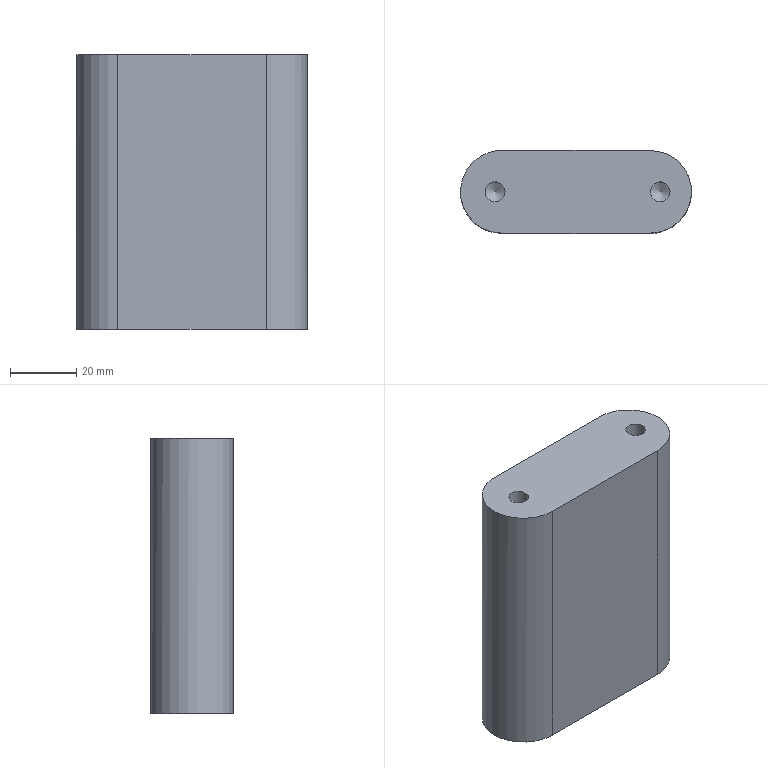Part | NX | features solid 2 | 1 solid | 10 faces | box 70.016 x 25 x 83 mm | volume 132398 mm3 | plane 4 | spline 2 | cone 2 | cylinder 2 | commonest cylinder face diameters 6 x2
STEP:
#1=CARTESIAN_POINT('',(542.,57.5,-33.));
#2=VERTEX_POINT('',#1);
#3=CARTESIAN_POINT('',(587.,57.5,-33.));
#4=VERTEX_POINT('',#3);
#5=CARTESIAN_POINT('',(542.,57.5,-33.));
#6=CARTESIAN_POINT('',(587.,57.5,-33.));
#7=B_SPLINE_CURVE_WITH_KNOTS('',1,(#5,#6),.UNSPECIFIED.,.F.,.F.,(2,2),(0.,1.),.PIECEWISE_BEZIER_KNOTS.);
#8=EDGE_CURVE('',#2,#4,#7,.T.);
#9=ORIENTED_EDGE('',*,*,#8,.F.);
#10=CARTESIAN_POINT('',(542.,57.5,50.));
#11=VERTEX_POINT('',#10);
#12=CARTESIAN_POINT('',(542.,57.5,20.));
#13=DIRECTION('',(0.,0.,-1.));
#14=VECTOR('',#13,1000.);
#15=LINE('',#12,#14);
#16=EDGE_CURVE('',#11,#2,#15,.T.);
#17=ORIENTED_EDGE('',*,*,#16,.F.);
#18=CARTESIAN_POINT('',(587.,57.5,50.));
#19=VERTEX_POINT('',#18);
#20=CARTESIAN_POINT('',(542.,57.5,50.));
#21=DIRECTION('',(1.,0.,0.));
#22=VECTOR('',#21,1000.);
#23=LINE('',#20,#22);
#24=EDGE_CURVE('',#11,#19,#23,.T.);
#25=ORIENTED_EDGE('',*,*,#24,.T.);
#26=CARTESIAN_POINT('',(587.,57.5,20.));
#27=DIRECTION('',(0.,0.,-1.));
#28=VECTOR('',#27,1000.);
#29=LINE('',#26,#28);
#30=EDGE_CURVE('',#19,#4,#29,.T.);
#31=ORIENTED_EDGE('',*,*,#30,.T.);
#32=EDGE_LOOP('',(#9,#17,#25,#31));
#33=FACE_BOUND('',#32,.T.);
#34=CARTESIAN_POINT('',(542.,57.5,20.));
#35=DIRECTION('',(0.,1.,0.));
#36=DIRECTION('',(0.,0.,1.));
#37=AXIS2_PLACEMENT_3D('',#34,#35,#36);
#38=PLANE('',#37);
#39=ADVANCED_FACE('',(#33),#38,.T.);
#40=CARTESIAN_POINT('',(587.,32.5,-33.));
#41=VERTEX_POINT('',#40);
#42=CARTESIAN_POINT('',(587.,57.5,-33.));
#43=CARTESIAN_POINT('',(588.638,57.5,-33.));
#44=CARTESIAN_POINT('',(591.905,56.833,-33.));
#45=CARTESIAN_POINT('',(596.086,54.084,-33.));
#46=CARTESIAN_POINT('',(598.837,49.907,-33.));
#47=CARTESIAN_POINT('',(599.843,45.,-33.));
#48=CARTESIAN_POINT('',(598.837,40.093,-33.));
#49=CARTESIAN_POINT('',(596.086,35.916,-33.));
#50=CARTESIAN_POINT('',(591.905,33.167,-33.));
#51=CARTESIAN_POINT('',(588.638,32.5,-33.));
#52=CARTESIAN_POINT('',(587.,32.5,-33.));
#53=B_SPLINE_CURVE_WITH_KNOTS('',3,(#42,#43,#44,#45,#46,#47,#48,#49,#50,#51,#52),.UNSPECIFIED.,.F.,.F.,(4,1,1,1,1,1,1,1,4),(0.,0.125,0.25,0.375,0.5,0.625,0.75,0.875,1.),.QUASI_UNIFORM_KNOTS.);
#54=EDGE_CURVE('',#4,#41,#53,.T.);
#55=ORIENTED_EDGE('',*,*,#54,.F.);
#56=ORIENTED_EDGE('',*,*,#30,.F.);
#57=CARTESIAN_POINT('',(587.,32.5,50.));
#58=VERTEX_POINT('',#57);
#59=CARTESIAN_POINT('',(587.,57.5,50.));
#60=CARTESIAN_POINT('',(590.258,57.5,50.));
#61=CARTESIAN_POINT('',(596.809,54.809,50.));
#62=CARTESIAN_POINT('',(600.858,45.002,50.));
#63=CARTESIAN_POINT('',(596.808,35.18,50.));
#64=CARTESIAN_POINT('',(590.24,32.5,50.));
#65=CARTESIAN_POINT('',(587.,32.5,50.));
#66=B_SPLINE_CURVE_WITH_KNOTS('',3,(#59,#60,#61,#62,#63,#64,#65),.UNSPECIFIED.,.F.,.F.,(4,1,1,1,4),(0.06855,0.07833,0.0881,0.09787,0.1076),.UNSPECIFIED.);
#67=EDGE_CURVE('',#19,#58,#66,.T.);
#68=ORIENTED_EDGE('',*,*,#67,.T.);
#69=CARTESIAN_POINT('',(587.,32.5,20.));
#70=DIRECTION('',(0.,0.,-1.));
#71=VECTOR('',#70,1000.);
#72=LINE('',#69,#71);
#73=EDGE_CURVE('',#58,#41,#72,.T.);
#74=ORIENTED_EDGE('',*,*,#73,.T.);
#75=EDGE_LOOP('',(#55,#56,#68,#74));
#76=FACE_BOUND('',#75,.T.);
#77=CARTESIAN_POINT('',(587.,57.5,50.));
#78=CARTESIAN_POINT('',(587.,57.5,-33.));
#79=CARTESIAN_POINT('',(590.276,57.5,50.));
#80=CARTESIAN_POINT('',(590.276,57.5,-33.));
#81=CARTESIAN_POINT('',(596.803,54.807,50.));
#82=CARTESIAN_POINT('',(596.803,54.807,-33.));
#83=CARTESIAN_POINT('',(600.86,45.,50.));
#84=CARTESIAN_POINT('',(600.86,45.,-33.));
#85=CARTESIAN_POINT('',(596.803,35.193,50.));
#86=CARTESIAN_POINT('',(596.803,35.193,-33.));
#87=CARTESIAN_POINT('',(590.276,32.5,50.));
#88=CARTESIAN_POINT('',(590.276,32.5,-33.));
#89=CARTESIAN_POINT('',(587.,32.5,50.));
#90=CARTESIAN_POINT('',(587.,32.5,-33.));
#91=B_SPLINE_SURFACE_WITH_KNOTS('',3,1,((#77,#78),(#79,#80),(#81,#82),(#83,#84),(#85,#86),(#87,#88),(#89,#90)),.SURF_OF_LINEAR_EXTRUSION.,.F.,.F.,.F.,(4,1,1,1,4),(2,2),(0.,0.25,0.5,0.75,1.),(0.,1.),.UNSPECIFIED.);
#92=ADVANCED_FACE('',(#76),#91,.T.);
#93=CARTESIAN_POINT('',(542.,32.5,-33.));
#94=VERTEX_POINT('',#93);
#95=CARTESIAN_POINT('',(587.,32.5,-33.));
#96=CARTESIAN_POINT('',(542.,32.5,-33.));
#97=B_SPLINE_CURVE_WITH_KNOTS('',1,(#95,#96),.UNSPECIFIED.,.F.,.F.,(2,2),(0.,1.),.PIECEWISE_BEZIER_KNOTS.);
#98=EDGE_CURVE('',#41,#94,#97,.T.);
#99=ORIENTED_EDGE('',*,*,#98,.F.);
#100=ORIENTED_EDGE('',*,*,#73,.F.);
#101=CARTESIAN_POINT('',(542.,32.5,50.));
#102=VERTEX_POINT('',#101);
#103=CARTESIAN_POINT('',(587.,32.5,50.));
#104=DIRECTION('',(-1.,0.,0.));
#105=VECTOR('',#104,1000.);
#106=LINE('',#103,#105);
#107=EDGE_CURVE('',#58,#102,#106,.T.);
#108=ORIENTED_EDGE('',*,*,#107,.T.);
#109=CARTESIAN_POINT('',(542.,32.5,20.));
#110=DIRECTION('',(0.,0.,-1.));
#111=VECTOR('',#110,1000.);
#112=LINE('',#109,#111);
#113=EDGE_CURVE('',#102,#94,#112,.T.);
#114=ORIENTED_EDGE('',*,*,#113,.T.);
#115=EDGE_LOOP('',(#99,#100,#108,#114));
#116=FACE_BOUND('',#115,.T.);
#117=CARTESIAN_POINT('',(587.,32.5,20.));
#118=DIRECTION('',(0.,-1.,0.));
#119=DIRECTION('',(0.,0.,-1.));
#120=AXIS2_PLACEMENT_3D('',#117,#118,#119);
#121=PLANE('',#120);
#122=ADVANCED_FACE('',(#116),#121,.T.);
#123=CARTESIAN_POINT('',(542.,32.5,-33.));
#124=CARTESIAN_POINT('',(540.362,32.5,-33.));
#125=CARTESIAN_POINT('',(537.095,33.167,-33.));
#126=CARTESIAN_POINT('',(532.914,35.916,-33.));
#127=CARTESIAN_POINT('',(530.163,40.093,-33.));
#128=CARTESIAN_POINT('',(529.157,45.,-33.));
#129=CARTESIAN_POINT('',(530.163,49.907,-33.));
#130=CARTESIAN_POINT('',(532.914,54.084,-33.));
#131=CARTESIAN_POINT('',(537.095,56.833,-33.));
#132=CARTESIAN_POINT('',(540.362,57.5,-33.));
#133=CARTESIAN_POINT('',(542.,57.5,-33.));
#134=B_SPLINE_CURVE_WITH_KNOTS('',3,(#123,#124,#125,#126,#127,#128,#129,#130,#131,#132,#133),.UNSPECIFIED.,.F.,.F.,(4,1,1,1,1,1,1,1,4),(0.,0.125,0.25,0.375,0.5,0.625,0.75,0.875,1.),.QUASI_UNIFORM_KNOTS.);
#135=EDGE_CURVE('',#94,#2,#134,.T.);
#136=ORIENTED_EDGE('',*,*,#135,.F.);
#137=ORIENTED_EDGE('',*,*,#113,.F.);
#138=CARTESIAN_POINT('',(542.,32.5,50.));
#139=CARTESIAN_POINT('',(538.695,32.5,50.));
#140=CARTESIAN_POINT('',(532.208,35.198,50.));
#141=CARTESIAN_POINT('',(528.138,44.985,50.));
#142=CARTESIAN_POINT('',(532.193,54.795,50.));
#143=CARTESIAN_POINT('',(538.696,57.5,50.));
#144=CARTESIAN_POINT('',(542.,57.5,50.));
#145=B_SPLINE_CURVE_WITH_KNOTS('',3,(#138,#139,#140,#141,#142,#143,#144),.UNSPECIFIED.,.F.,.F.,(4,1,1,1,4),(0.,0.009769,0.01954,0.02931,0.03908),.UNSPECIFIED.);
#146=EDGE_CURVE('',#102,#11,#145,.T.);
#147=ORIENTED_EDGE('',*,*,#146,.T.);
#148=ORIENTED_EDGE('',*,*,#16,.T.);
#149=EDGE_LOOP('',(#136,#137,#147,#148));
#150=FACE_BOUND('',#149,.T.);
#151=CARTESIAN_POINT('',(542.,32.5,50.));
#152=CARTESIAN_POINT('',(542.,32.5,-33.));
#153=CARTESIAN_POINT('',(538.724,32.5,50.));
#154=CARTESIAN_POINT('',(538.724,32.5,-33.));
#155=CARTESIAN_POINT('',(532.197,35.193,50.));
#156=CARTESIAN_POINT('',(532.197,35.193,-33.));
#157=CARTESIAN_POINT('',(528.14,45.,50.));
#158=CARTESIAN_POINT('',(528.14,45.,-33.));
#159=CARTESIAN_POINT('',(532.197,54.807,50.));
#160=CARTESIAN_POINT('',(532.197,54.807,-33.));
#161=CARTESIAN_POINT('',(538.724,57.5,50.));
#162=CARTESIAN_POINT('',(538.724,57.5,-33.));
#163=CARTESIAN_POINT('',(542.,57.5,50.));
#164=CARTESIAN_POINT('',(542.,57.5,-33.));
#165=B_SPLINE_SURFACE_WITH_KNOTS('',3,1,((#151,#152),(#153,#154),(#155,#156),(#157,#158),(#159,#160),(#161,#162),(#163,#164)),.SURF_OF_LINEAR_EXTRUSION.,.F.,.F.,.F.,(4,1,1,1,4),(2,2),(0.,0.25,0.5,0.75,1.),(0.,1.),.UNSPECIFIED.);
#166=ADVANCED_FACE('',(#150),#165,.T.);
#167=CARTESIAN_POINT('',(543.,45.,50.));
#168=VERTEX_POINT('',#167);
#169=CARTESIAN_POINT('',(540.,45.,50.));
#170=DIRECTION('',(0.,0.,1.));
#171=DIRECTION('',(1.,0.,0.));
#172=AXIS2_PLACEMENT_3D('',#169,#170,#171);
#173=CIRCLE('',#172,3.);
#174=EDGE_CURVE('',#168,#168,#173,.F.);
#175=ORIENTED_EDGE('',*,*,#174,.T.);
#176=EDGE_LOOP('',(#175));
#177=FACE_BOUND('',#176,.T.);
#178=CARTESIAN_POINT('',(593.,45.,50.));
#179=VERTEX_POINT('',#178);
#180=CARTESIAN_POINT('',(590.,45.,50.));
#181=DIRECTION('',(0.,0.,1.));
#182=DIRECTION('',(1.,0.,0.));
#183=AXIS2_PLACEMENT_3D('',#180,#181,#182);
#184=CIRCLE('',#183,3.);
#185=EDGE_CURVE('',#179,#179,#184,.F.);
#186=ORIENTED_EDGE('',*,*,#185,.T.);
#187=EDGE_LOOP('',(#186));
#188=FACE_BOUND('',#187,.T.);
#189=ORIENTED_EDGE('',*,*,#24,.F.);
#190=ORIENTED_EDGE('',*,*,#146,.F.);
#191=ORIENTED_EDGE('',*,*,#107,.F.);
#192=ORIENTED_EDGE('',*,*,#67,.F.);
#193=EDGE_LOOP('',(#189,#190,#191,#192));
#194=FACE_BOUND('',#193,.T.);
#195=CARTESIAN_POINT('',(599.508,45.,50.));
#196=DIRECTION('',(0.,0.,1.));
#197=DIRECTION('',(1.,0.,0.));
#198=AXIS2_PLACEMENT_3D('',#195,#196,#197);
#199=PLANE('',#198);
#200=ADVANCED_FACE('',(#177,#188,#194),#199,.T.);
#201=ORIENTED_EDGE('',*,*,#8,.T.);
#202=ORIENTED_EDGE('',*,*,#54,.T.);
#203=ORIENTED_EDGE('',*,*,#98,.T.);
#204=ORIENTED_EDGE('',*,*,#135,.T.);
#205=EDGE_LOOP('',(#201,#202,#203,#204));
#206=FACE_BOUND('',#205,.T.);
#207=CARTESIAN_POINT('',(599.508,45.,-33.));
#208=DIRECTION('',(0.,0.,1.));
#209=DIRECTION('',(1.,0.,0.));
#210=AXIS2_PLACEMENT_3D('',#207,#208,#209);
#211=PLANE('',#210);
#212=ADVANCED_FACE('',(#206),#211,.F.);
#213=CARTESIAN_POINT('',(593.,45.,20.399));
#214=VERTEX_POINT('',#213);
#215=CARTESIAN_POINT('',(590.,45.,20.399));
#216=DIRECTION('',(0.,0.,1.));
#217=DIRECTION('',(1.,0.,0.));
#218=AXIS2_PLACEMENT_3D('',#215,#216,#217);
#219=CIRCLE('',#218,3.);
#220=EDGE_CURVE('',#214,#214,#219,.F.);
#221=ORIENTED_EDGE('',*,*,#220,.F.);
#222=EDGE_LOOP('',(#221));
#223=FACE_BOUND('',#222,.T.);
#224=CARTESIAN_POINT('',(590.,45.,18.597));
#225=VERTEX_POINT('',#224);
#226=VERTEX_LOOP('',#225);
#227=FACE_BOUND('',#226,.T.);
#228=CARTESIAN_POINT('',(590.,45.,21.));
#229=DIRECTION('',(0.,0.,1.));
#230=DIRECTION('',(1.,0.,0.));
#231=AXIS2_PLACEMENT_3D('',#228,#229,#230);
#232=CONICAL_SURFACE('',#231,4.,1.03);
#233=ADVANCED_FACE('',(#223,#227),#232,.F.);
#234=ORIENTED_EDGE('',*,*,#220,.T.);
#235=EDGE_LOOP('',(#234));
#236=FACE_BOUND('',#235,.T.);
#237=ORIENTED_EDGE('',*,*,#185,.F.);
#238=EDGE_LOOP('',(#237));
#239=FACE_BOUND('',#238,.T.);
#240=CARTESIAN_POINT('',(590.,45.,50.));
#241=DIRECTION('',(0.,0.,-1.));
#242=DIRECTION('',(-1.,0.,0.));
#243=AXIS2_PLACEMENT_3D('',#240,#241,#242);
#244=CYLINDRICAL_SURFACE('',#243,3.);
#245=ADVANCED_FACE('',(#236,#239),#244,.F.);
#246=CARTESIAN_POINT('',(543.,45.,20.399));
#247=VERTEX_POINT('',#246);
#248=CARTESIAN_POINT('',(540.,45.,20.399));
#249=DIRECTION('',(0.,0.,1.));
#250=DIRECTION('',(1.,0.,0.));
#251=AXIS2_PLACEMENT_3D('',#248,#249,#250);
#252=CIRCLE('',#251,3.);
#253=EDGE_CURVE('',#247,#247,#252,.F.);
#254=ORIENTED_EDGE('',*,*,#253,.F.);
#255=EDGE_LOOP('',(#254));
#256=FACE_BOUND('',#255,.T.);
#257=CARTESIAN_POINT('',(540.,45.,18.597));
#258=VERTEX_POINT('',#257);
#259=VERTEX_LOOP('',#258);
#260=FACE_BOUND('',#259,.T.);
#261=CARTESIAN_POINT('',(540.,45.,21.));
#262=DIRECTION('',(0.,0.,1.));
#263=DIRECTION('',(1.,0.,0.));
#264=AXIS2_PLACEMENT_3D('',#261,#262,#263);
#265=CONICAL_SURFACE('',#264,4.,1.03);
#266=ADVANCED_FACE('',(#256,#260),#265,.F.);
#267=ORIENTED_EDGE('',*,*,#253,.T.);
#268=EDGE_LOOP('',(#267));
#269=FACE_BOUND('',#268,.T.);
#270=ORIENTED_EDGE('',*,*,#174,.F.);
#271=EDGE_LOOP('',(#270));
#272=FACE_BOUND('',#271,.T.);
#273=CARTESIAN_POINT('',(540.,45.,50.));
#274=DIRECTION('',(0.,0.,-1.));
#275=DIRECTION('',(-1.,0.,0.));
#276=AXIS2_PLACEMENT_3D('',#273,#274,#275);
#277=CYLINDRICAL_SURFACE('',#276,3.);
#278=ADVANCED_FACE('',(#269,#272),#277,.F.);
#279=CLOSED_SHELL('',(#39,#92,#122,#166,#200,#212,#233,#245,#266,#278));
#280=MANIFOLD_SOLID_BREP('',#279);
#281=(LENGTH_UNIT()NAMED_UNIT(*)SI_UNIT(.MILLI.,.METRE.));
#282=UNCERTAINTY_MEASURE_WITH_UNIT(LENGTH_MEASURE(0.0508),#281,'','');
#283=(NAMED_UNIT(*)PLANE_ANGLE_UNIT()SI_UNIT($,.RADIAN.));
#284=(NAMED_UNIT(*)SI_UNIT($,.STERADIAN.)SOLID_ANGLE_UNIT());
#285=(GEOMETRIC_REPRESENTATION_CONTEXT(3)GLOBAL_UNCERTAINTY_ASSIGNED_CONTEXT((#282))GLOBAL_UNIT_ASSIGNED_CONTEXT((#281,#283,#284))REPRESENTATION_CONTEXT('',''));
#286=ADVANCED_BREP_SHAPE_REPRESENTATION('',(#280),#285);